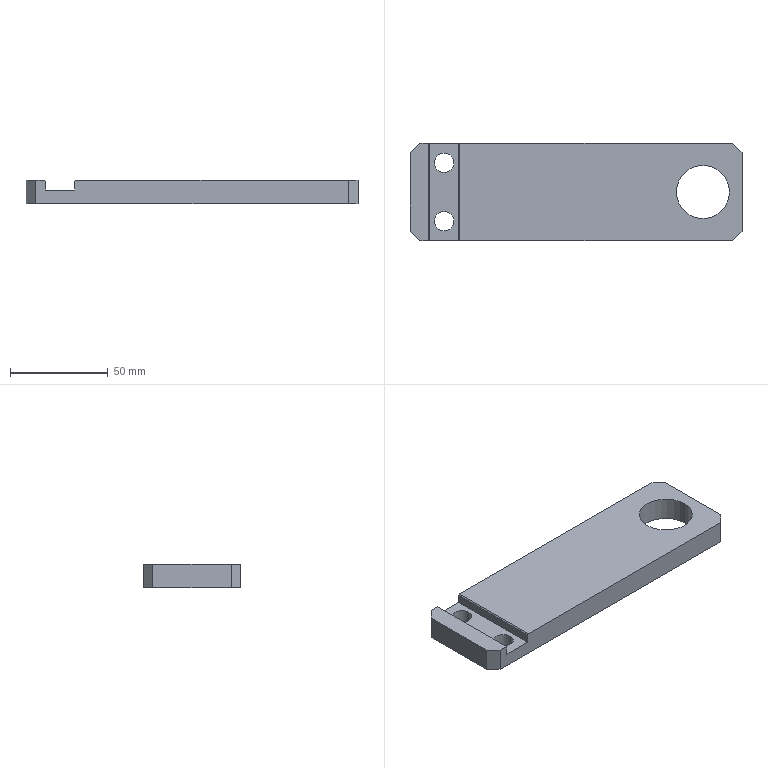Part | STEP file | [01]-12 | 1 solid | 22 faces | box 170 x 50 x 12 mm | volume 89565 mm3 | plane 16 | cylinder 6 | commonest cylinder face diameters 10 x4 27.2 x2